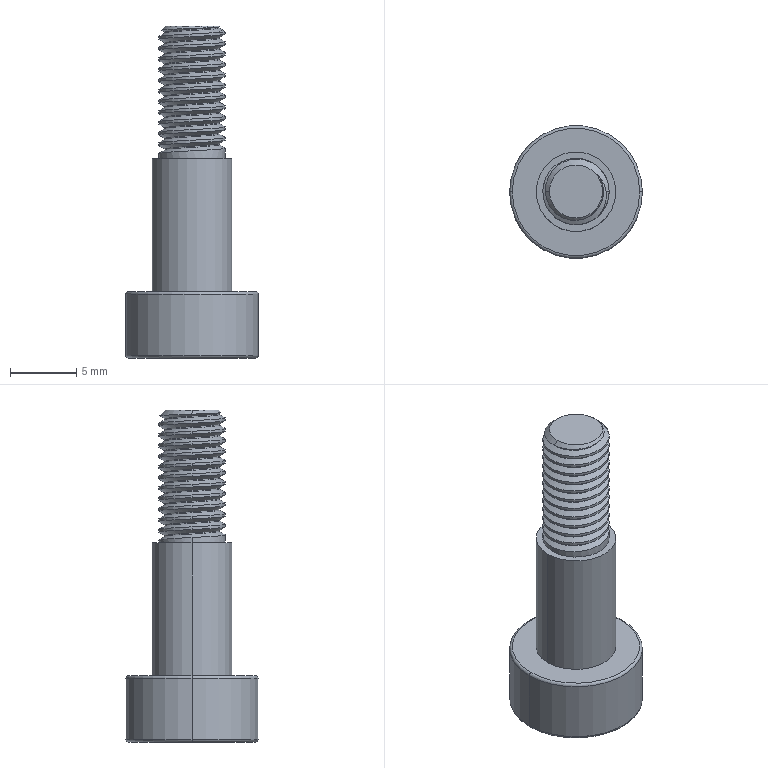Part | SolidWorks | features ICE 3, Chamfer 1, Extrusion 1, Fillet 1, SweepThread 1 | 1 solid | 53 faces | box 10 x 10 x 25 mm | volume 739.596 mm3 | cylinder 29 | plane 14 | torus 4 | cone 3 | spline 3 | commonest cylinder face diameters 5 x25 6 x2 10 x2